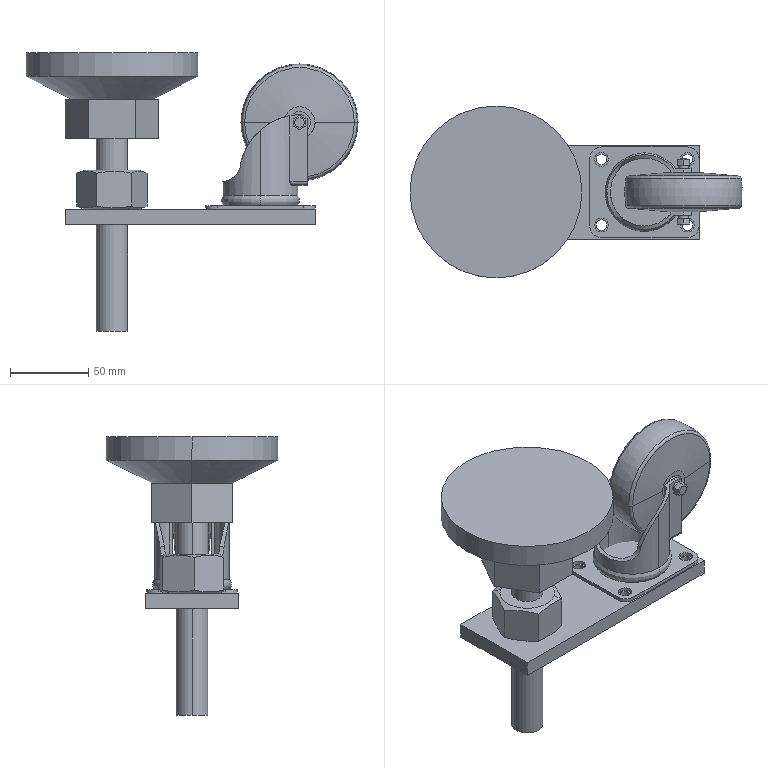Part | SolidWorks | 3 solids | 138 faces | box 212.5 x 110 x 178 mm | volume 375386 mm3 | cylinder 57 | plane 57 | torus 16 | cone 8 | commonest cylinder face diameters 6.8 x8 8.8 x8 20 x8 6 x4 9.98 x4 13.98 x4